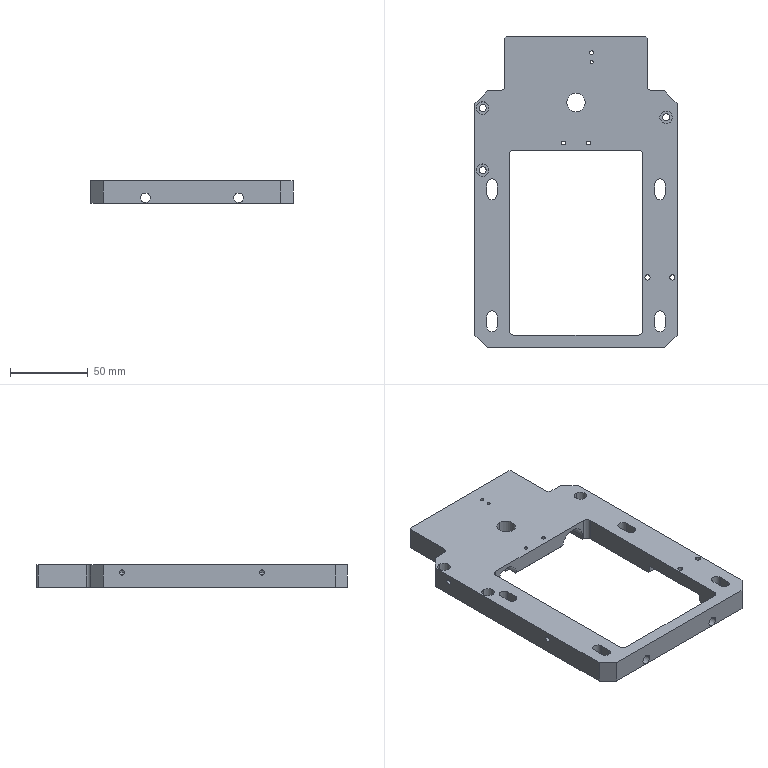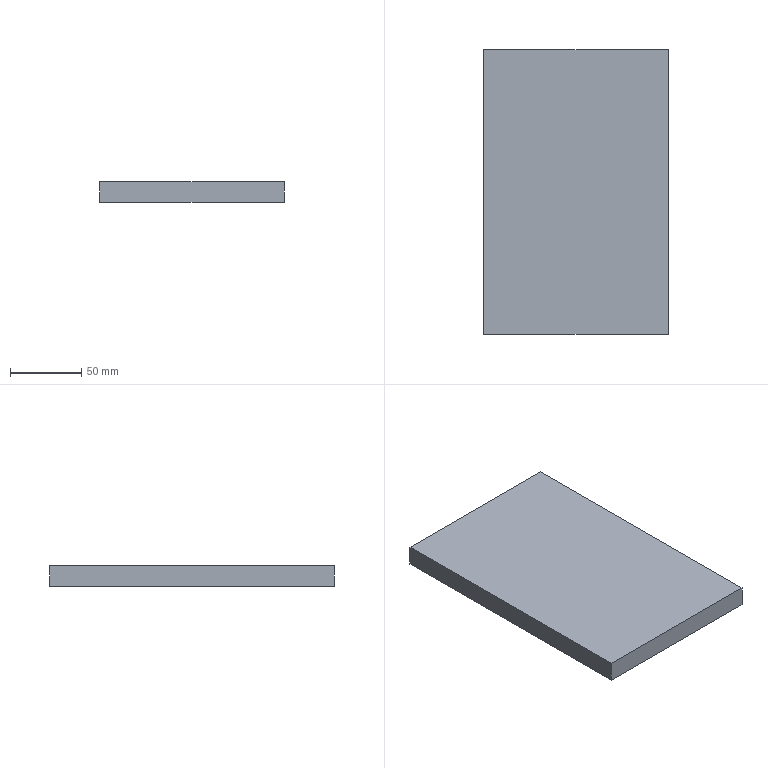CAM job | NX | 3+2 milling, drilling | part box 130 x 200 x 14.5 mm | stock box 130 x 200 x 14.5 mm
Tools:
number,name,description,diameter,corner_radius,flute_length,length,flutes
21,ZXZ,Milling Tool-5 Parameters,6.0,0.0,50.0,75.0,2
12,4.5ZT,Drilling Tool,4.5,0.0,35.0,50.0,2
13,3.3ZT,Drilling Tool,3.3,0.0,35.0,50.0,2
22,2.5ZT,Drilling Tool,2.5,0.0,35.0,50.0,2
24,1.6ZT,Drilling Tool,1.6,0.0,35.0,50.0,2
4,D10,Milling Tool-5 Parameters,10.0,0.0,50.0,75.0,2
17,D4,Milling Tool-5 Parameters,4.0,0.0,50.0,75.0,2
6,D6,Milling Tool-5 Parameters,6.0,0.0,50.0,75.0,2
16,D6JING,Milling Tool-5 Parameters,6.0,0.0,50.0,75.0,2
9,R2,Milling Tool-5 Parameters,4.0,2.0,50.0,75.0,2
19,D1.5,Milling Tool-5 Parameters,1.5,0.0,50.0,75.0,2
1,D6A45,Milling Tool-5 Parameters,6.0,0.0,50.0,75.0,2
18,D2,Milling Tool-5 Parameters,2.0,0.0,50.0,75.0,2
23,2.1ZT,Drilling Tool,2.05,0.0,35.0,50.0,2
Operations:
program,operation,operation_type,tool,method,geometry_group,spindle_rpm,surface_speed,feed_per_tooth,feed_cut,feed_plunge,cut_length_mm,path_length_mm,cut_time_min,machine_time_min
1,DRILLING,Operation,ZXZ,METHOD,A,3500.0,65.0,0.0357,250.0,0.0,48.0,574.166,0.192,0.2446
1,DRILLING_COPY,Operation,4.5ZT,METHOD,A,2000.0,28.0,0.0375,150.0,0.0,75.408,378.954,0.5027,0.5331
1,DRILLING_COPY_1,Operation,3.3ZT,METHOD,A,2000.0,21.0,0.0375,150.0,0.0,39.983,159.244,0.2666,0.2785
1,DRILLING_COPY_COPY,Operation,2.5ZT,METHOD,A,2000.0,21.0,0.0375,150.0,0.0,59.253,261.588,0.395,0.4153
1,DRILLING_COPY_1_COPY,Operation,1.6ZT,METHOD,A,2000.0,37.0,0.025,100.0,0.0,19.481,98.961,0.1948,0.2028
1,DRILLING_COPY_1_COPY_COPY,Operation,2.1ZT,METHOD,A,2000.0,37.0,0.025,100.0,0.0,22.602,116.748,0.226,0.2354
1,ZLEVEL_PROFILE_1_COPY,ZLevelMilling,D10,METHOD,A,3500.0,109.0,0.3143,2200.0,1000.0,20925.168,20996.518,9.529,9.536
1,ZLEVEL_PROFILE_1,ZLevelMilling,D10,METHOD,A,3500.0,109.0,0.3143,2200.0,1000.0,26627.647,26698.997,12.121,12.128
1,ZLEVEL_PROFILE,ZLevelMilling,D10,METHOD,A,3500.0,109.0,0.3143,2200.0,1000.0,13023.458,13811.332,6.294,6.373
1,FLOOR_WALL,VolumeBased25DMillingOperation,D10,METHOD,A,3500.0,109.0,0.3571,2500.0,1000.0,8884.748,10652.968,3.906,4.083
1,ZLEVEL_PROFILE_COPY,ZLevelMilling,D10,METHOD,A,3500.0,109.0,0.3143,2200.0,1000.0,15837.942,16238.622,7.205,7.245
1,HOLE_MILLING,CylinderMilling,D10,METHOD,A,3500.0,0.0,0.0,2000.0,100.0,416.209,490.209,0.2081,0.2155
1,ZLEVEL_PROFILE_1_COPY_1,ZLevelMilling,D6,METHOD,A,4000.0,75.0,0.225,1800.0,1000.0,7715.837,8238.298,4.341,4.393
1,ZLEVEL_PROFILE_COPY_COPY,ZLevelMilling,D4,METHOD,A,5500.0,69.0,0.15,1650.0,1000.0,4049.294,4483.446,2.456,2.499
1,ZLEVEL_PROFILE_COPY_COPY_COPY,ZLevelMilling,D4,METHOD,A,5500.0,69.0,0.15,1650.0,1000.0,6482.627,10679.592,4.307,4.727
1,ZLEVEL_PROFILE_1_COPY_1_COPY,ZLevelMilling,D4,METHOD,A,6000.0,75.0,0.1125,1350.0,1000.0,8886.96,9477.569,6.614,6.673
1,FLOOR_WALL_1_COPY,VolumeBased25DMillingOperation,D6JING,METHOD,A,7500.0,235.0,0.08,1200.0,1000.0,720.42,1239.843,0.602,0.654
1,FLOOR_WALL_1_COPY_COPY,VolumeBased25DMillingOperation,D6JING,METHOD,A,7500.0,235.0,0.08,1200.0,1000.0,134.832,700.052,0.1137,0.1702
1,ZLEVEL_PROFILE_2,ZLevelMilling,D6JING,METHOD,A,7500.0,235.0,0.0667,1000.0,100.0,391.865,478.565,0.3919,0.4005
1,ZLEVEL_PROFILE_2_COPY,ZLevelMilling,D6JING,METHOD,A,7500.0,235.0,0.0667,1000.0,100.0,205.756,1160.222,0.2058,0.3012
1,FIXED_CONTOUR,SurfaceContour,R2,METHOD,A,7500.0,94.0,0.1867,2800.0,1000.0,41528.802,41865.252,14.853,14.887
1,HOLE_MILLING_1,CylinderMilling,D1.5,METHOD,A,6000.0,28.0,0.0833,1000.0,100.0,1415.917,1489.917,1.416,1.423
1,PLANAR_MILL,PlanarMilling,D6A45,METHOD,A,7500.0,141.0,0.0833,1250.0,100.0,1511.372,2577.687,1.209,1.316
1,PLANAR_MILL_COPY,PlanarMilling,D6A45,METHOD,A,7500.0,141.0,0.0833,1250.0,100.0,47.745,112.745,0.0382,0.0447
1,刀补19,CylinderMilling,D1.5,METHOD,A,6000.0,28.0,0.0667,800.0,100.0,224.142,298.142,0.2802,0.2876
2,HOLE_MILLING_COPY,CylinderMilling,D6,METHOD,B,5500.0,103.0,0.1364,1500.0,100.0,1366.762,1727.863,0.9112,0.9473
2,PLANAR_MILL_COPY_1,PlanarMilling,D6A45,METHOD,B,7500.0,141.0,0.0833,1250.0,100.0,1355.863,2887.748,1.085,1.238
3,DRILLING_COPY_2,Operation,ZXZ,METHOD,C,3500.0,65.0,0.0357,250.0,0.0,16.0,273.781,0.064,0.0898
3,DRILLING_COPY_1_COPY_1,Operation,3.3ZT,METHOD,C,2000.0,21.0,0.0375,150.0,0.0,36.183,165.515,0.2412,0.2542
3,DRILLING_COPY_COPY_COPY,Operation,2.5ZT,METHOD,C,2000.0,21.0,0.0375,150.0,0.0,16.0,180.053,0.1067,0.1231
3,HOLE_MILLING_2,CylinderMilling,D2,METHOD,C,7500.0,47.0,0.0533,800.0,100.0,1308.269,1522.269,1.635,1.657
3,DRILLING_COPY_2_COPY,Operation,D6A45,METHOD,C,3500.0,65.0,0.0357,250.0,0.0,18.4,278.581,0.0736,0.0996
3,刀补18,CylinderMilling,D2,METHOD,C,7500.0,47.0,0.0533,800.0,100.0,43.977,257.977,0.055,0.0764